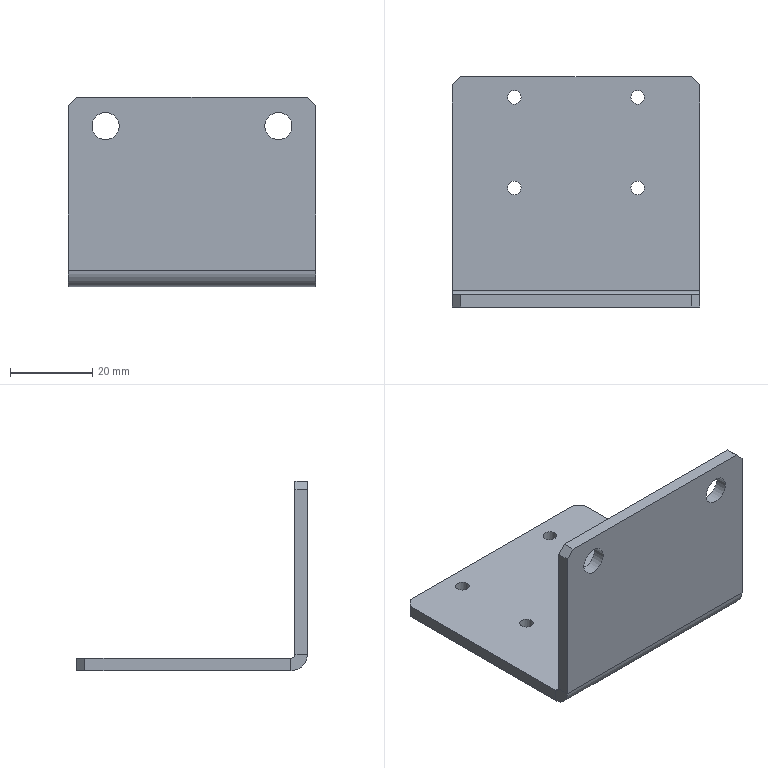Part | NX | 1 solid | 24 faces | box 60 x 56 x 46 mm | volume 17295 mm3 | plane 16 | cylinder 8 | commonest cylinder face diameters 3.3 x4 6.6 x2 2 x1 8 x1
STEP:
#1=CARTESIAN_POINT('',(30.,-25.5,-3.));
#2=VERTEX_POINT('',#1);
#3=CARTESIAN_POINT('',(30.,24.5,-3.));
#4=VERTEX_POINT('',#3);
#5=CARTESIAN_POINT('',(30.,-26.5,-3.));
#6=DIRECTION('',(0.,1.,0.));
#7=VECTOR('',#6,1000.);
#8=LINE('',#5,#7);
#9=EDGE_CURVE('',#2,#4,#8,.T.);
#10=ORIENTED_EDGE('',*,*,#9,.T.);
#11=CARTESIAN_POINT('',(30.,24.5,0.));
#12=VERTEX_POINT('',#11);
#13=CARTESIAN_POINT('',(30.,24.5,-3.));
#14=DIRECTION('',(0.,0.,1.));
#15=VECTOR('',#14,1000.);
#16=LINE('',#13,#15);
#17=EDGE_CURVE('',#4,#12,#16,.T.);
#18=ORIENTED_EDGE('',*,*,#17,.T.);
#19=CARTESIAN_POINT('',(30.,-25.5,0.));
#20=VERTEX_POINT('',#19);
#21=CARTESIAN_POINT('',(30.,-26.5,0.));
#22=DIRECTION('',(0.,1.,0.));
#23=VECTOR('',#22,1000.);
#24=LINE('',#21,#23);
#25=EDGE_CURVE('',#20,#12,#24,.T.);
#26=ORIENTED_EDGE('',*,*,#25,.F.);
#27=CARTESIAN_POINT('',(30.,-25.5,0.));
#28=DIRECTION('',(0.,0.,-1.));
#29=VECTOR('',#28,1000.);
#30=LINE('',#27,#29);
#31=EDGE_CURVE('',#20,#2,#30,.T.);
#32=ORIENTED_EDGE('',*,*,#31,.T.);
#33=EDGE_LOOP('',(#10,#18,#26,#32));
#34=FACE_BOUND('',#33,.T.);
#35=CARTESIAN_POINT('',(30.,-26.5,-3.));
#36=DIRECTION('',(1.,0.,0.));
#37=DIRECTION('',(0.,0.,-1.));
#38=AXIS2_PLACEMENT_3D('',#35,#36,#37);
#39=PLANE('',#38);
#40=ADVANCED_FACE('',(#34),#39,.T.);
#41=CARTESIAN_POINT('',(-16.65,-0.5,-3.));
#42=VERTEX_POINT('',#41);
#43=CARTESIAN_POINT('',(-15.,-0.5,-3.));
#44=DIRECTION('',(0.,0.,-1.));
#45=DIRECTION('',(-1.,0.,0.));
#46=AXIS2_PLACEMENT_3D('',#43,#44,#45);
#47=CIRCLE('',#46,1.65);
#48=EDGE_CURVE('',#42,#42,#47,.T.);
#49=ORIENTED_EDGE('',*,*,#48,.F.);
#50=EDGE_LOOP('',(#49));
#51=FACE_BOUND('',#50,.T.);
#52=CARTESIAN_POINT('',(-16.65,21.5,-3.));
#53=VERTEX_POINT('',#52);
#54=CARTESIAN_POINT('',(-15.,21.5,-3.));
#55=DIRECTION('',(0.,0.,-1.));
#56=DIRECTION('',(-1.,0.,0.));
#57=AXIS2_PLACEMENT_3D('',#54,#55,#56);
#58=CIRCLE('',#57,1.65);
#59=EDGE_CURVE('',#53,#53,#58,.T.);
#60=ORIENTED_EDGE('',*,*,#59,.F.);
#61=EDGE_LOOP('',(#60));
#62=FACE_BOUND('',#61,.T.);
#63=CARTESIAN_POINT('',(13.35,-0.5,-3.));
#64=VERTEX_POINT('',#63);
#65=CARTESIAN_POINT('',(15.,-0.5,-3.));
#66=DIRECTION('',(0.,0.,-1.));
#67=DIRECTION('',(-1.,0.,0.));
#68=AXIS2_PLACEMENT_3D('',#65,#66,#67);
#69=CIRCLE('',#68,1.65);
#70=EDGE_CURVE('',#64,#64,#69,.T.);
#71=ORIENTED_EDGE('',*,*,#70,.F.);
#72=EDGE_LOOP('',(#71));
#73=FACE_BOUND('',#72,.T.);
#74=CARTESIAN_POINT('',(13.35,21.5,-3.));
#75=VERTEX_POINT('',#74);
#76=CARTESIAN_POINT('',(15.,21.5,-3.));
#77=DIRECTION('',(0.,0.,-1.));
#78=DIRECTION('',(-1.,0.,0.));
#79=AXIS2_PLACEMENT_3D('',#76,#77,#78);
#80=CIRCLE('',#79,1.65);
#81=EDGE_CURVE('',#75,#75,#80,.T.);
#82=ORIENTED_EDGE('',*,*,#81,.F.);
#83=EDGE_LOOP('',(#82));
#84=FACE_BOUND('',#83,.T.);
#85=CARTESIAN_POINT('',(28.,26.5,-3.));
#86=VERTEX_POINT('',#85);
#87=CARTESIAN_POINT('',(-28.,26.5,-3.));
#88=VERTEX_POINT('',#87);
#89=CARTESIAN_POINT('',(-30.,26.5,-3.));
#90=DIRECTION('',(-1.,0.,0.));
#91=VECTOR('',#90,1000.);
#92=LINE('',#89,#91);
#93=EDGE_CURVE('',#86,#88,#92,.T.);
#94=ORIENTED_EDGE('',*,*,#93,.F.);
#95=CARTESIAN_POINT('',(27.25,27.25,-3.));
#96=DIRECTION('',(-0.7071,0.7071,0.));
#97=VECTOR('',#96,1000.);
#98=LINE('',#95,#97);
#99=EDGE_CURVE('',#86,#4,#98,.F.);
#100=ORIENTED_EDGE('',*,*,#99,.T.);
#101=ORIENTED_EDGE('',*,*,#9,.F.);
#102=CARTESIAN_POINT('',(-30.,-25.5,-3.));
#103=VERTEX_POINT('',#102);
#104=CARTESIAN_POINT('',(30.,-25.5,-3.));
#105=DIRECTION('',(1.,0.,0.));
#106=VECTOR('',#105,1000.);
#107=LINE('',#104,#106);
#108=EDGE_CURVE('',#2,#103,#107,.F.);
#109=ORIENTED_EDGE('',*,*,#108,.T.);
#110=CARTESIAN_POINT('',(-30.,24.5,-3.));
#111=VERTEX_POINT('',#110);
#112=CARTESIAN_POINT('',(-30.,-26.5,-3.));
#113=DIRECTION('',(0.,-1.,0.));
#114=VECTOR('',#113,1000.);
#115=LINE('',#112,#114);
#116=EDGE_CURVE('',#111,#103,#115,.T.);
#117=ORIENTED_EDGE('',*,*,#116,.F.);
#118=CARTESIAN_POINT('',(-27.25,27.25,-3.));
#119=DIRECTION('',(-0.7071,-0.7071,0.));
#120=VECTOR('',#119,1000.);
#121=LINE('',#118,#120);
#122=EDGE_CURVE('',#111,#88,#121,.F.);
#123=ORIENTED_EDGE('',*,*,#122,.T.);
#124=EDGE_LOOP('',(#94,#100,#101,#109,#117,#123));
#125=FACE_BOUND('',#124,.T.);
#126=CARTESIAN_POINT('',(0.,0.,-3.));
#127=DIRECTION('',(0.,0.,-1.));
#128=DIRECTION('',(-1.,0.,0.));
#129=AXIS2_PLACEMENT_3D('',#126,#127,#128);
#130=PLANE('',#129);
#131=ADVANCED_FACE('',(#51,#62,#73,#84,#125),#130,.T.);
#132=CARTESIAN_POINT('',(-16.65,-0.5,0.));
#133=VERTEX_POINT('',#132);
#134=CARTESIAN_POINT('',(-15.,-0.5,0.));
#135=DIRECTION('',(0.,0.,-1.));
#136=DIRECTION('',(-1.,0.,0.));
#137=AXIS2_PLACEMENT_3D('',#134,#135,#136);
#138=CIRCLE('',#137,1.65);
#139=EDGE_CURVE('',#133,#133,#138,.T.);
#140=ORIENTED_EDGE('',*,*,#139,.T.);
#141=EDGE_LOOP('',(#140));
#142=FACE_BOUND('',#141,.T.);
#143=CARTESIAN_POINT('',(-16.65,21.5,0.));
#144=VERTEX_POINT('',#143);
#145=CARTESIAN_POINT('',(-15.,21.5,0.));
#146=DIRECTION('',(0.,0.,-1.));
#147=DIRECTION('',(-1.,0.,0.));
#148=AXIS2_PLACEMENT_3D('',#145,#146,#147);
#149=CIRCLE('',#148,1.65);
#150=EDGE_CURVE('',#144,#144,#149,.T.);
#151=ORIENTED_EDGE('',*,*,#150,.T.);
#152=EDGE_LOOP('',(#151));
#153=FACE_BOUND('',#152,.T.);
#154=CARTESIAN_POINT('',(13.35,-0.5,0.));
#155=VERTEX_POINT('',#154);
#156=CARTESIAN_POINT('',(15.,-0.5,0.));
#157=DIRECTION('',(0.,0.,-1.));
#158=DIRECTION('',(-1.,0.,0.));
#159=AXIS2_PLACEMENT_3D('',#156,#157,#158);
#160=CIRCLE('',#159,1.65);
#161=EDGE_CURVE('',#155,#155,#160,.T.);
#162=ORIENTED_EDGE('',*,*,#161,.T.);
#163=EDGE_LOOP('',(#162));
#164=FACE_BOUND('',#163,.T.);
#165=CARTESIAN_POINT('',(13.35,21.5,0.));
#166=VERTEX_POINT('',#165);
#167=CARTESIAN_POINT('',(15.,21.5,0.));
#168=DIRECTION('',(0.,0.,-1.));
#169=DIRECTION('',(-1.,0.,0.));
#170=AXIS2_PLACEMENT_3D('',#167,#168,#169);
#171=CIRCLE('',#170,1.65);
#172=EDGE_CURVE('',#166,#166,#171,.T.);
#173=ORIENTED_EDGE('',*,*,#172,.T.);
#174=EDGE_LOOP('',(#173));
#175=FACE_BOUND('',#174,.T.);
#176=ORIENTED_EDGE('',*,*,#25,.T.);
#177=CARTESIAN_POINT('',(28.,26.5,0.));
#178=VERTEX_POINT('',#177);
#179=CARTESIAN_POINT('',(30.,24.5,0.));
#180=DIRECTION('',(0.7071,-0.7071,0.));
#181=VECTOR('',#180,1000.);
#182=LINE('',#179,#181);
#183=EDGE_CURVE('',#12,#178,#182,.F.);
#184=ORIENTED_EDGE('',*,*,#183,.T.);
#185=CARTESIAN_POINT('',(-28.,26.5,0.));
#186=VERTEX_POINT('',#185);
#187=CARTESIAN_POINT('',(-30.,26.5,0.));
#188=DIRECTION('',(-1.,0.,0.));
#189=VECTOR('',#188,1000.);
#190=LINE('',#187,#189);
#191=EDGE_CURVE('',#178,#186,#190,.T.);
#192=ORIENTED_EDGE('',*,*,#191,.T.);
#193=CARTESIAN_POINT('',(-30.,24.5,0.));
#194=VERTEX_POINT('',#193);
#195=CARTESIAN_POINT('',(-28.,26.5,0.));
#196=DIRECTION('',(0.7071,0.7071,0.));
#197=VECTOR('',#196,1000.);
#198=LINE('',#195,#197);
#199=EDGE_CURVE('',#186,#194,#198,.F.);
#200=ORIENTED_EDGE('',*,*,#199,.T.);
#201=CARTESIAN_POINT('',(-30.,-25.5,0.));
#202=VERTEX_POINT('',#201);
#203=CARTESIAN_POINT('',(-30.,-26.5,0.));
#204=DIRECTION('',(0.,-1.,0.));
#205=VECTOR('',#204,1000.);
#206=LINE('',#203,#205);
#207=EDGE_CURVE('',#194,#202,#206,.T.);
#208=ORIENTED_EDGE('',*,*,#207,.T.);
#209=CARTESIAN_POINT('',(30.,-25.5,0.));
#210=DIRECTION('',(1.,0.,0.));
#211=VECTOR('',#210,1000.);
#212=LINE('',#209,#211);
#213=EDGE_CURVE('',#20,#202,#212,.F.);
#214=ORIENTED_EDGE('',*,*,#213,.F.);
#215=EDGE_LOOP('',(#176,#184,#192,#200,#208,#214));
#216=FACE_BOUND('',#215,.T.);
#217=CARTESIAN_POINT('',(0.,0.,0.));
#218=DIRECTION('',(0.,0.,-1.));
#219=DIRECTION('',(-1.,0.,0.));
#220=AXIS2_PLACEMENT_3D('',#217,#218,#219);
#221=PLANE('',#220);
#222=ADVANCED_FACE('',(#142,#153,#164,#175,#216),#221,.F.);
#223=ORIENTED_EDGE('',*,*,#207,.F.);
#224=CARTESIAN_POINT('',(-30.,24.5,-3.));
#225=DIRECTION('',(0.,0.,-1.));
#226=VECTOR('',#225,1000.);
#227=LINE('',#224,#226);
#228=EDGE_CURVE('',#194,#111,#227,.T.);
#229=ORIENTED_EDGE('',*,*,#228,.T.);
#230=ORIENTED_EDGE('',*,*,#116,.T.);
#231=CARTESIAN_POINT('',(-30.,-25.5,0.));
#232=DIRECTION('',(0.,0.,-1.));
#233=VECTOR('',#232,1000.);
#234=LINE('',#231,#233);
#235=EDGE_CURVE('',#202,#103,#234,.T.);
#236=ORIENTED_EDGE('',*,*,#235,.F.);
#237=EDGE_LOOP('',(#223,#229,#230,#236));
#238=FACE_BOUND('',#237,.T.);
#239=CARTESIAN_POINT('',(-30.,-26.5,-3.));
#240=DIRECTION('',(-1.,0.,0.));
#241=DIRECTION('',(0.,0.,1.));
#242=AXIS2_PLACEMENT_3D('',#239,#240,#241);
#243=PLANE('',#242);
#244=ADVANCED_FACE('',(#238),#243,.T.);
#245=ORIENTED_EDGE('',*,*,#191,.F.);
#246=CARTESIAN_POINT('',(28.,26.5,-3.));
#247=DIRECTION('',(0.,0.,-1.));
#248=VECTOR('',#247,1000.);
#249=LINE('',#246,#248);
#250=EDGE_CURVE('',#178,#86,#249,.T.);
#251=ORIENTED_EDGE('',*,*,#250,.T.);
#252=ORIENTED_EDGE('',*,*,#93,.T.);
#253=CARTESIAN_POINT('',(-28.,26.5,-3.));
#254=DIRECTION('',(0.,0.,1.));
#255=VECTOR('',#254,1000.);
#256=LINE('',#253,#255);
#257=EDGE_CURVE('',#88,#186,#256,.T.);
#258=ORIENTED_EDGE('',*,*,#257,.T.);
#259=EDGE_LOOP('',(#245,#251,#252,#258));
#260=FACE_BOUND('',#259,.T.);
#261=CARTESIAN_POINT('',(-30.,26.5,-3.));
#262=DIRECTION('',(0.,1.,0.));
#263=DIRECTION('',(0.,0.,1.));
#264=AXIS2_PLACEMENT_3D('',#261,#262,#263);
#265=PLANE('',#264);
#266=ADVANCED_FACE('',(#260),#265,.T.);
#267=ORIENTED_EDGE('',*,*,#139,.F.);
#268=EDGE_LOOP('',(#267));
#269=FACE_BOUND('',#268,.T.);
#270=ORIENTED_EDGE('',*,*,#48,.T.);
#271=EDGE_LOOP('',(#270));
#272=FACE_BOUND('',#271,.T.);
#273=CARTESIAN_POINT('',(-15.,-0.5,-3.));
#274=DIRECTION('',(0.,0.,-1.));
#275=DIRECTION('',(-1.,0.,0.));
#276=AXIS2_PLACEMENT_3D('',#273,#274,#275);
#277=CYLINDRICAL_SURFACE('',#276,1.65);
#278=ADVANCED_FACE('',(#269,#272),#277,.F.);
#279=ORIENTED_EDGE('',*,*,#150,.F.);
#280=EDGE_LOOP('',(#279));
#281=FACE_BOUND('',#280,.T.);
#282=ORIENTED_EDGE('',*,*,#59,.T.);
#283=EDGE_LOOP('',(#282));
#284=FACE_BOUND('',#283,.T.);
#285=CARTESIAN_POINT('',(-15.,21.5,-3.));
#286=DIRECTION('',(0.,0.,-1.));
#287=DIRECTION('',(-1.,0.,0.));
#288=AXIS2_PLACEMENT_3D('',#285,#286,#287);
#289=CYLINDRICAL_SURFACE('',#288,1.65);
#290=ADVANCED_FACE('',(#281,#284),#289,.F.);
#291=ORIENTED_EDGE('',*,*,#161,.F.);
#292=EDGE_LOOP('',(#291));
#293=FACE_BOUND('',#292,.T.);
#294=ORIENTED_EDGE('',*,*,#70,.T.);
#295=EDGE_LOOP('',(#294));
#296=FACE_BOUND('',#295,.T.);
#297=CARTESIAN_POINT('',(15.,-0.5,-3.));
#298=DIRECTION('',(0.,0.,-1.));
#299=DIRECTION('',(-1.,0.,0.));
#300=AXIS2_PLACEMENT_3D('',#297,#298,#299);
#301=CYLINDRICAL_SURFACE('',#300,1.65);
#302=ADVANCED_FACE('',(#293,#296),#301,.F.);
#303=ORIENTED_EDGE('',*,*,#172,.F.);
#304=EDGE_LOOP('',(#303));
#305=FACE_BOUND('',#304,.T.);
#306=ORIENTED_EDGE('',*,*,#81,.T.);
#307=EDGE_LOOP('',(#306));
#308=FACE_BOUND('',#307,.T.);
#309=CARTESIAN_POINT('',(15.,21.5,-3.));
#310=DIRECTION('',(0.,0.,-1.));
#311=DIRECTION('',(-1.,0.,0.));
#312=AXIS2_PLACEMENT_3D('',#309,#310,#311);
#313=CYLINDRICAL_SURFACE('',#312,1.65);
#314=ADVANCED_FACE('',(#305,#308),#313,.F.);
#315=CARTESIAN_POINT('',(-30.,-26.5,1.));
#316=VERTEX_POINT('',#315);
#317=CARTESIAN_POINT('',(-30.,-29.5,1.));
#318=VERTEX_POINT('',#317);
#319=CARTESIAN_POINT('',(-30.,-26.5,1.));
#320=DIRECTION('',(0.,-1.,0.));
#321=VECTOR('',#320,1000.);
#322=LINE('',#319,#321);
#323=EDGE_CURVE('',#316,#318,#322,.T.);
#324=ORIENTED_EDGE('',*,*,#323,.F.);
#325=CARTESIAN_POINT('',(-30.,-25.5,1.));
#326=DIRECTION('',(1.,0.,0.));
#327=DIRECTION('',(0.,0.,-1.));
#328=AXIS2_PLACEMENT_3D('',#325,#326,#327);
#329=CIRCLE('',#328,1.);
#330=EDGE_CURVE('',#202,#316,#329,.F.);
#331=ORIENTED_EDGE('',*,*,#330,.F.);
#332=ORIENTED_EDGE('',*,*,#235,.T.);
#333=CARTESIAN_POINT('',(-30.,-25.5,1.));
#334=DIRECTION('',(1.,0.,0.));
#335=DIRECTION('',(0.,0.,-1.));
#336=AXIS2_PLACEMENT_3D('',#333,#334,#335);
#337=CIRCLE('',#336,4.);
#338=EDGE_CURVE('',#103,#318,#337,.F.);
#339=ORIENTED_EDGE('',*,*,#338,.T.);
#340=EDGE_LOOP('',(#324,#331,#332,#339));
#341=FACE_BOUND('',#340,.T.);
#342=CARTESIAN_POINT('',(-30.,-25.5,1.));
#343=DIRECTION('',(-1.,0.,0.));
#344=DIRECTION('',(0.,0.,1.));
#345=AXIS2_PLACEMENT_3D('',#342,#343,#344);
#346=PLANE('',#345);
#347=ADVANCED_FACE('',(#341),#346,.T.);
#348=CARTESIAN_POINT('',(30.,-26.5,1.));
#349=VERTEX_POINT('',#348);
#350=CARTESIAN_POINT('',(30.,-25.5,1.));
#351=DIRECTION('',(1.,0.,0.));
#352=DIRECTION('',(0.,0.,-1.));
#353=AXIS2_PLACEMENT_3D('',#350,#351,#352);
#354=CIRCLE('',#353,1.);
#355=EDGE_CURVE('',#349,#20,#354,.T.);
#356=ORIENTED_EDGE('',*,*,#355,.F.);
#357=CARTESIAN_POINT('',(30.,-29.5,1.));
#358=VERTEX_POINT('',#357);
#359=CARTESIAN_POINT('',(30.,-26.5,1.));
#360=DIRECTION('',(0.,-1.,0.));
#361=VECTOR('',#360,1000.);
#362=LINE('',#359,#361);
#363=EDGE_CURVE('',#349,#358,#362,.T.);
#364=ORIENTED_EDGE('',*,*,#363,.T.);
#365=CARTESIAN_POINT('',(30.,-25.5,1.));
#366=DIRECTION('',(1.,0.,0.));
#367=DIRECTION('',(0.,0.,-1.));
#368=AXIS2_PLACEMENT_3D('',#365,#366,#367);
#369=CIRCLE('',#368,4.);
#370=EDGE_CURVE('',#358,#2,#369,.T.);
#371=ORIENTED_EDGE('',*,*,#370,.T.);
#372=ORIENTED_EDGE('',*,*,#31,.F.);
#373=EDGE_LOOP('',(#356,#364,#371,#372));
#374=FACE_BOUND('',#373,.T.);
#375=CARTESIAN_POINT('',(30.,-25.5,1.));
#376=DIRECTION('',(-1.,0.,0.));
#377=DIRECTION('',(0.,0.,1.));
#378=AXIS2_PLACEMENT_3D('',#375,#376,#377);
#379=PLANE('',#378);
#380=ADVANCED_FACE('',(#374),#379,.F.);
#381=ORIENTED_EDGE('',*,*,#108,.F.);
#382=ORIENTED_EDGE('',*,*,#370,.F.);
#383=CARTESIAN_POINT('',(0.,-29.5,1.));
#384=DIRECTION('',(-1.,0.,0.));
#385=VECTOR('',#384,1000.);
#386=LINE('',#383,#385);
#387=EDGE_CURVE('',#358,#318,#386,.T.);
#388=ORIENTED_EDGE('',*,*,#387,.T.);
#389=ORIENTED_EDGE('',*,*,#338,.F.);
#390=EDGE_LOOP('',(#381,#382,#388,#389));
#391=FACE_BOUND('',#390,.T.);
#392=CARTESIAN_POINT('',(30.,-25.5,1.));
#393=DIRECTION('',(1.,0.,0.));
#394=DIRECTION('',(0.,-1.,0.));
#395=AXIS2_PLACEMENT_3D('',#392,#393,#394);
#396=CYLINDRICAL_SURFACE('',#395,4.);
#397=ADVANCED_FACE('',(#391),#396,.T.);
#398=ORIENTED_EDGE('',*,*,#213,.T.);
#399=ORIENTED_EDGE('',*,*,#330,.T.);
#400=CARTESIAN_POINT('',(-30.,-26.5,1.));
#401=DIRECTION('',(1.,0.,0.));
#402=VECTOR('',#401,1000.);
#403=LINE('',#400,#402);
#404=EDGE_CURVE('',#316,#349,#403,.T.);
#405=ORIENTED_EDGE('',*,*,#404,.T.);
#406=ORIENTED_EDGE('',*,*,#355,.T.);
#407=EDGE_LOOP('',(#398,#399,#405,#406));
#408=FACE_BOUND('',#407,.T.);
#409=CARTESIAN_POINT('',(30.,-25.5,1.));
#410=DIRECTION('',(1.,0.,0.));
#411=DIRECTION('',(0.,-1.,0.));
#412=AXIS2_PLACEMENT_3D('',#409,#410,#411);
#413=CYLINDRICAL_SURFACE('',#412,1.);
#414=ADVANCED_FACE('',(#408),#413,.F.);
#415=CARTESIAN_POINT('',(30.,-26.5,41.));
#416=VERTEX_POINT('',#415);
#417=CARTESIAN_POINT('',(30.,-26.5,43.));
#418=DIRECTION('',(0.,0.,1.));
#419=VECTOR('',#418,1000.);
#420=LINE('',#417,#419);
#421=EDGE_CURVE('',#349,#416,#420,.T.);
#422=ORIENTED_EDGE('',*,*,#421,.T.);
#423=CARTESIAN_POINT('',(30.,-29.5,41.));
#424=VERTEX_POINT('',#423);
#425=CARTESIAN_POINT('',(30.,-29.5,41.));
#426=DIRECTION('',(0.,-1.,0.));
#427=VECTOR('',#426,1000.);
#428=LINE('',#425,#427);
#429=EDGE_CURVE('',#416,#424,#428,.T.);
#430=ORIENTED_EDGE('',*,*,#429,.T.);
#431=CARTESIAN_POINT('',(30.,-29.5,43.));
#432=DIRECTION('',(0.,0.,1.));
#433=VECTOR('',#432,1000.);
#434=LINE('',#431,#433);
#435=EDGE_CURVE('',#358,#424,#434,.T.);
#436=ORIENTED_EDGE('',*,*,#435,.F.);
#437=ORIENTED_EDGE('',*,*,#363,.F.);
#438=EDGE_LOOP('',(#422,#430,#436,#437));
#439=FACE_BOUND('',#438,.T.);
#440=CARTESIAN_POINT('',(30.,-29.5,43.));
#441=DIRECTION('',(-1.,0.,0.));
#442=DIRECTION('',(0.,0.,1.));
#443=AXIS2_PLACEMENT_3D('',#440,#441,#442);
#444=PLANE('',#443);
#445=ADVANCED_FACE('',(#439),#444,.F.);
#446=CARTESIAN_POINT('',(-30.,-29.5,41.));
#447=VERTEX_POINT('',#446);
#448=CARTESIAN_POINT('',(-30.,-29.5,0.));
#449=DIRECTION('',(0.,0.,-1.));
#450=VECTOR('',#449,1000.);
#451=LINE('',#448,#450);
#452=EDGE_CURVE('',#447,#318,#451,.T.);
#453=ORIENTED_EDGE('',*,*,#452,.F.);
#454=CARTESIAN_POINT('',(-30.,-26.5,41.));
#455=VERTEX_POINT('',#454);
#456=CARTESIAN_POINT('',(-30.,-29.5,41.));
#457=DIRECTION('',(0.,1.,0.));
#458=VECTOR('',#457,1000.);
#459=LINE('',#456,#458);
#460=EDGE_CURVE('',#447,#455,#459,.T.);
#461=ORIENTED_EDGE('',*,*,#460,.T.);
#462=CARTESIAN_POINT('',(-30.,-26.5,0.));
#463=DIRECTION('',(0.,0.,-1.));
#464=VECTOR('',#463,1000.);
#465=LINE('',#462,#464);
#466=EDGE_CURVE('',#455,#316,#465,.T.);
#467=ORIENTED_EDGE('',*,*,#466,.T.);
#468=ORIENTED_EDGE('',*,*,#323,.T.);
#469=EDGE_LOOP('',(#453,#461,#467,#468));
#470=FACE_BOUND('',#469,.T.);
#471=CARTESIAN_POINT('',(-30.,-29.5,0.));
#472=DIRECTION('',(1.,0.,0.));
#473=DIRECTION('',(0.,0.,-1.));
#474=AXIS2_PLACEMENT_3D('',#471,#472,#473);
#475=PLANE('',#474);
#476=ADVANCED_FACE('',(#470),#475,.F.);
#477=CARTESIAN_POINT('',(-21.,-29.5,32.7));
#478=VERTEX_POINT('',#477);
#479=CARTESIAN_POINT('',(-21.,-29.5,36.));
#480=DIRECTION('',(0.,-1.,0.));
#481=DIRECTION('',(0.,0.,-1.));
#482=AXIS2_PLACEMENT_3D('',#479,#480,#481);
#483=CIRCLE('',#482,3.3);
#484=EDGE_CURVE('',#478,#478,#483,.T.);
#485=ORIENTED_EDGE('',*,*,#484,.F.);
#486=EDGE_LOOP('',(#485));
#487=FACE_BOUND('',#486,.T.);
#488=CARTESIAN_POINT('',(21.,-29.5,32.7));
#489=VERTEX_POINT('',#488);
#490=CARTESIAN_POINT('',(21.,-29.5,36.));
#491=DIRECTION('',(0.,-1.,0.));
#492=DIRECTION('',(0.,0.,-1.));
#493=AXIS2_PLACEMENT_3D('',#490,#491,#492);
#494=CIRCLE('',#493,3.3);
#495=EDGE_CURVE('',#489,#489,#494,.T.);
#496=ORIENTED_EDGE('',*,*,#495,.F.);
#497=EDGE_LOOP('',(#496));
#498=FACE_BOUND('',#497,.T.);
#499=CARTESIAN_POINT('',(28.,-29.5,43.));
#500=VERTEX_POINT('',#499);
#501=CARTESIAN_POINT('',(-28.,-29.5,43.));
#502=VERTEX_POINT('',#501);
#503=CARTESIAN_POINT('',(-30.,-29.5,43.));
#504=DIRECTION('',(-1.,0.,0.));
#505=VECTOR('',#504,1000.);
#506=LINE('',#503,#505);
#507=EDGE_CURVE('',#500,#502,#506,.T.);
#508=ORIENTED_EDGE('',*,*,#507,.T.);
#509=CARTESIAN_POINT('',(-30.,-29.5,41.));
#510=DIRECTION('',(0.7071,0.,0.7071));
#511=VECTOR('',#510,1000.);
#512=LINE('',#509,#511);
#513=EDGE_CURVE('',#502,#447,#512,.F.);
#514=ORIENTED_EDGE('',*,*,#513,.T.);
#515=ORIENTED_EDGE('',*,*,#452,.T.);
#516=ORIENTED_EDGE('',*,*,#387,.F.);
#517=ORIENTED_EDGE('',*,*,#435,.T.);
#518=CARTESIAN_POINT('',(28.,-29.5,43.));
#519=DIRECTION('',(0.7071,0.,-0.7071));
#520=VECTOR('',#519,1000.);
#521=LINE('',#518,#520);
#522=EDGE_CURVE('',#424,#500,#521,.F.);
#523=ORIENTED_EDGE('',*,*,#522,.T.);
#524=EDGE_LOOP('',(#508,#514,#515,#516,#517,#523));
#525=FACE_BOUND('',#524,.T.);
#526=CARTESIAN_POINT('',(0.,-29.5,0.));
#527=DIRECTION('',(0.,1.,0.));
#528=DIRECTION('',(0.,0.,1.));
#529=AXIS2_PLACEMENT_3D('',#526,#527,#528);
#530=PLANE('',#529);
#531=ADVANCED_FACE('',(#487,#498,#525),#530,.F.);
#532=CARTESIAN_POINT('',(-21.,-26.5,39.3));
#533=VERTEX_POINT('',#532);
#534=CARTESIAN_POINT('',(-21.,-26.5,36.));
#535=DIRECTION('',(0.,1.,0.));
#536=DIRECTION('',(0.,0.,1.));
#537=AXIS2_PLACEMENT_3D('',#534,#535,#536);
#538=CIRCLE('',#537,3.3);
#539=EDGE_CURVE('',#533,#533,#538,.T.);
#540=ORIENTED_EDGE('',*,*,#539,.F.);
#541=EDGE_LOOP('',(#540));
#542=FACE_BOUND('',#541,.T.);
#543=CARTESIAN_POINT('',(21.,-26.5,39.3));
#544=VERTEX_POINT('',#543);
#545=CARTESIAN_POINT('',(21.,-26.5,36.));
#546=DIRECTION('',(0.,1.,0.));
#547=DIRECTION('',(0.,0.,1.));
#548=AXIS2_PLACEMENT_3D('',#545,#546,#547);
#549=CIRCLE('',#548,3.3);
#550=EDGE_CURVE('',#544,#544,#549,.T.);
#551=ORIENTED_EDGE('',*,*,#550,.F.);
#552=EDGE_LOOP('',(#551));
#553=FACE_BOUND('',#552,.T.);
#554=ORIENTED_EDGE('',*,*,#466,.F.);
#555=CARTESIAN_POINT('',(-28.,-26.5,43.));
#556=VERTEX_POINT('',#555);
#557=CARTESIAN_POINT('',(-35.5,-26.5,35.5));
#558=DIRECTION('',(-0.7071,0.,-0.7071));
#559=VECTOR('',#558,1000.);
#560=LINE('',#557,#559);
#561=EDGE_CURVE('',#455,#556,#560,.F.);
#562=ORIENTED_EDGE('',*,*,#561,.T.);
#563=CARTESIAN_POINT('',(28.,-26.5,43.));
#564=VERTEX_POINT('',#563);
#565=CARTESIAN_POINT('',(-30.,-26.5,43.));
#566=DIRECTION('',(-1.,0.,0.));
#567=VECTOR('',#566,1000.);
#568=LINE('',#565,#567);
#569=EDGE_CURVE('',#564,#556,#568,.T.);
#570=ORIENTED_EDGE('',*,*,#569,.F.);
#571=CARTESIAN_POINT('',(35.5,-26.5,35.5));
#572=DIRECTION('',(-0.7071,0.,0.7071));
#573=VECTOR('',#572,1000.);
#574=LINE('',#571,#573);
#575=EDGE_CURVE('',#564,#416,#574,.F.);
#576=ORIENTED_EDGE('',*,*,#575,.T.);
#577=ORIENTED_EDGE('',*,*,#421,.F.);
#578=ORIENTED_EDGE('',*,*,#404,.F.);
#579=EDGE_LOOP('',(#554,#562,#570,#576,#577,#578));
#580=FACE_BOUND('',#579,.T.);
#581=CARTESIAN_POINT('',(0.,-26.5,0.));
#582=DIRECTION('',(0.,1.,0.));
#583=DIRECTION('',(0.,0.,1.));
#584=AXIS2_PLACEMENT_3D('',#581,#582,#583);
#585=PLANE('',#584);
#586=ADVANCED_FACE('',(#542,#553,#580),#585,.T.);
#587=ORIENTED_EDGE('',*,*,#569,.T.);
#588=CARTESIAN_POINT('',(-28.,-29.5,43.));
#589=DIRECTION('',(0.,-1.,0.));
#590=VECTOR('',#589,1000.);
#591=LINE('',#588,#590);
#592=EDGE_CURVE('',#556,#502,#591,.T.);
#593=ORIENTED_EDGE('',*,*,#592,.T.);
#594=ORIENTED_EDGE('',*,*,#507,.F.);
#595=CARTESIAN_POINT('',(28.,-29.5,43.));
#596=DIRECTION('',(0.,1.,0.));
#597=VECTOR('',#596,1000.);
#598=LINE('',#595,#597);
#599=EDGE_CURVE('',#500,#564,#598,.T.);
#600=ORIENTED_EDGE('',*,*,#599,.T.);
#601=EDGE_LOOP('',(#587,#593,#594,#600));
#602=FACE_BOUND('',#601,.T.);
#603=CARTESIAN_POINT('',(-30.,-29.5,43.));
#604=DIRECTION('',(0.,0.,-1.));
#605=DIRECTION('',(0.,1.,0.));
#606=AXIS2_PLACEMENT_3D('',#603,#604,#605);
#607=PLANE('',#606);
#608=ADVANCED_FACE('',(#602),#607,.F.);
#609=ORIENTED_EDGE('',*,*,#99,.F.);
#610=ORIENTED_EDGE('',*,*,#250,.F.);
#611=ORIENTED_EDGE('',*,*,#183,.F.);
#612=ORIENTED_EDGE('',*,*,#17,.F.);
#613=EDGE_LOOP('',(#609,#610,#611,#612));
#614=FACE_BOUND('',#613,.T.);
#615=CARTESIAN_POINT('',(30.,24.5,-3.));
#616=DIRECTION('',(-0.7071,-0.7071,0.));
#617=DIRECTION('',(0.,0.,1.));
#618=AXIS2_PLACEMENT_3D('',#615,#616,#617);
#619=PLANE('',#618);
#620=ADVANCED_FACE('',(#614),#619,.F.);
#621=ORIENTED_EDGE('',*,*,#122,.F.);
#622=ORIENTED_EDGE('',*,*,#228,.F.);
#623=ORIENTED_EDGE('',*,*,#199,.F.);
#624=ORIENTED_EDGE('',*,*,#257,.F.);
#625=EDGE_LOOP('',(#621,#622,#623,#624));
#626=FACE_BOUND('',#625,.T.);
#627=CARTESIAN_POINT('',(-28.,26.5,-3.));
#628=DIRECTION('',(0.7071,-0.7071,0.));
#629=DIRECTION('',(0.,0.,1.));
#630=AXIS2_PLACEMENT_3D('',#627,#628,#629);
#631=PLANE('',#630);
#632=ADVANCED_FACE('',(#626),#631,.F.);
#633=ORIENTED_EDGE('',*,*,#513,.F.);
#634=ORIENTED_EDGE('',*,*,#592,.F.);
#635=ORIENTED_EDGE('',*,*,#561,.F.);
#636=ORIENTED_EDGE('',*,*,#460,.F.);
#637=EDGE_LOOP('',(#633,#634,#635,#636));
#638=FACE_BOUND('',#637,.T.);
#639=CARTESIAN_POINT('',(-30.,-29.5,41.));
#640=DIRECTION('',(0.7071,0.,-0.7071));
#641=DIRECTION('',(0.,1.,0.));
#642=AXIS2_PLACEMENT_3D('',#639,#640,#641);
#643=PLANE('',#642);
#644=ADVANCED_FACE('',(#638),#643,.F.);
#645=ORIENTED_EDGE('',*,*,#522,.F.);
#646=ORIENTED_EDGE('',*,*,#429,.F.);
#647=ORIENTED_EDGE('',*,*,#575,.F.);
#648=ORIENTED_EDGE('',*,*,#599,.F.);
#649=EDGE_LOOP('',(#645,#646,#647,#648));
#650=FACE_BOUND('',#649,.T.);
#651=CARTESIAN_POINT('',(28.,-29.5,43.));
#652=DIRECTION('',(-0.7071,0.,-0.7071));
#653=DIRECTION('',(0.,1.,0.));
#654=AXIS2_PLACEMENT_3D('',#651,#652,#653);
#655=PLANE('',#654);
#656=ADVANCED_FACE('',(#650),#655,.F.);
#657=ORIENTED_EDGE('',*,*,#550,.T.);
#658=EDGE_LOOP('',(#657));
#659=FACE_BOUND('',#658,.T.);
#660=ORIENTED_EDGE('',*,*,#495,.T.);
#661=EDGE_LOOP('',(#660));
#662=FACE_BOUND('',#661,.T.);
#663=CARTESIAN_POINT('',(21.,-29.5,36.));
#664=DIRECTION('',(0.,-1.,0.));
#665=DIRECTION('',(0.,0.,-1.));
#666=AXIS2_PLACEMENT_3D('',#663,#664,#665);
#667=CYLINDRICAL_SURFACE('',#666,3.3);
#668=ADVANCED_FACE('',(#659,#662),#667,.F.);
#669=ORIENTED_EDGE('',*,*,#539,.T.);
#670=EDGE_LOOP('',(#669));
#671=FACE_BOUND('',#670,.T.);
#672=ORIENTED_EDGE('',*,*,#484,.T.);
#673=EDGE_LOOP('',(#672));
#674=FACE_BOUND('',#673,.T.);
#675=CARTESIAN_POINT('',(-21.,-29.5,36.));
#676=DIRECTION('',(0.,-1.,0.));
#677=DIRECTION('',(0.,0.,-1.));
#678=AXIS2_PLACEMENT_3D('',#675,#676,#677);
#679=CYLINDRICAL_SURFACE('',#678,3.3);
#680=ADVANCED_FACE('',(#671,#674),#679,.F.);
#681=CLOSED_SHELL('',(#40,#131,#222,#244,#266,#278,#290,#302,#314,#347,#380,#397,#414,#445,#476,#531,#586,#608,#620,#632,#644,#656,#668,#680));
#682=MANIFOLD_SOLID_BREP('',#681);
#683=(LENGTH_UNIT()NAMED_UNIT(*)SI_UNIT(.MILLI.,.METRE.));
#684=UNCERTAINTY_MEASURE_WITH_UNIT(LENGTH_MEASURE(0.00001),#683,'','');
#685=(NAMED_UNIT(*)PLANE_ANGLE_UNIT()SI_UNIT($,.RADIAN.));
#686=(NAMED_UNIT(*)SI_UNIT($,.STERADIAN.)SOLID_ANGLE_UNIT());
#687=(GEOMETRIC_REPRESENTATION_CONTEXT(3)GLOBAL_UNCERTAINTY_ASSIGNED_CONTEXT((#684))GLOBAL_UNIT_ASSIGNED_CONTEXT((#683,#685,#686))REPRESENTATION_CONTEXT('',''));
#688=ADVANCED_BREP_SHAPE_REPRESENTATION('',(#682),#687);